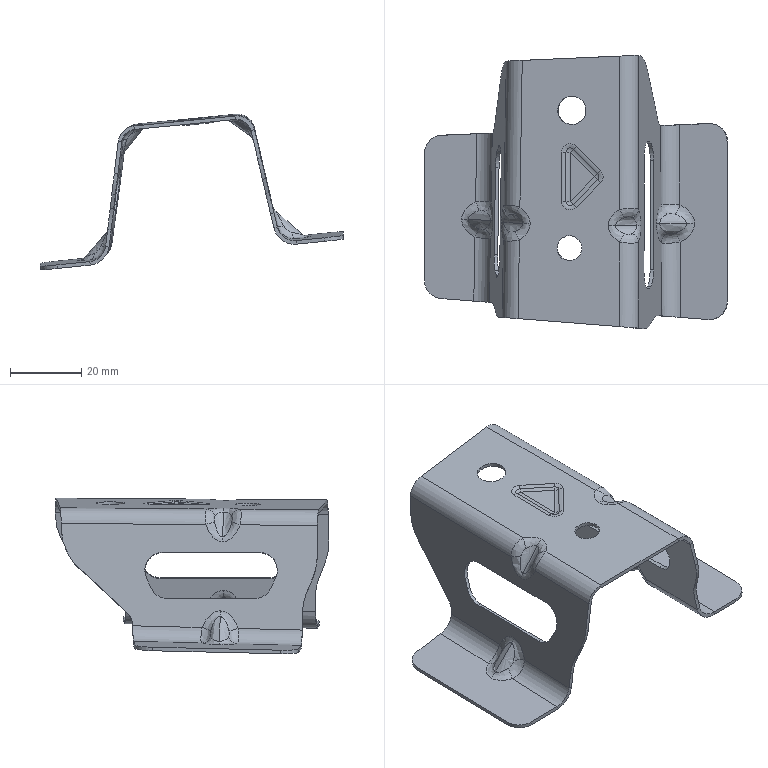Part | 1 solid | 176 faces | box 85.103 x 76.79 x 43.71 mm | volume 7815 mm3 | spline 116 | cylinder 32 | plane 15 | sphere 6 | other 4 | torus 3 | commonest cylinder face diameters 8 x9 10 x8 6 x6 12 x4 4 x3 7 x2